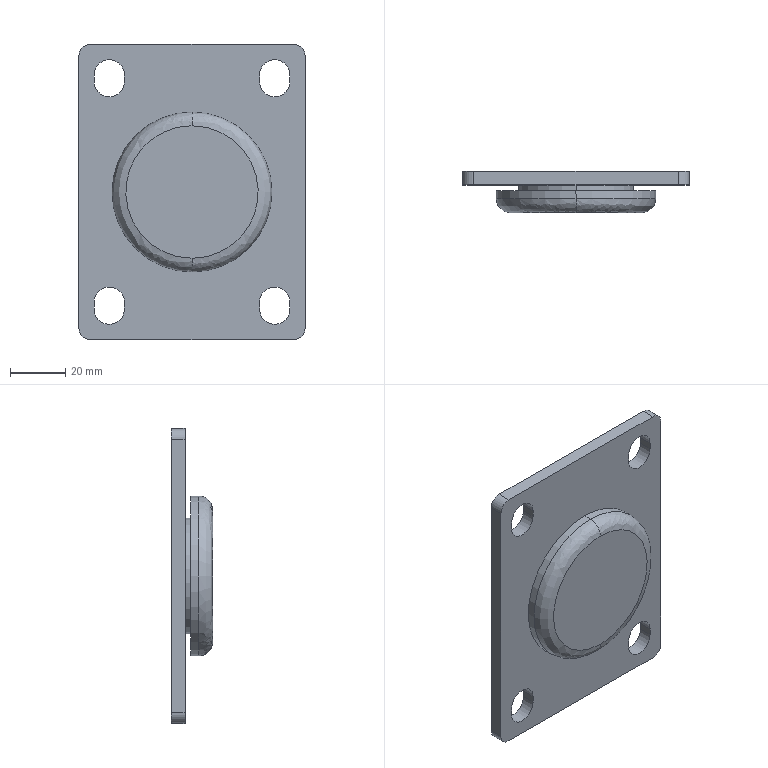Part | SolidWorks | features BaseBody 1 | 1 solid | 47 faces | box 82 x 15 x 107 mm | volume 61600 mm3 | cylinder 26 | plane 19 | spline 2 | commonest cylinder face diameters 11 x12 8 x4 25 x2 40 x2 42 x2 58 x2
STEP:
#1=CARTESIAN_POINT('',(0.,49.,-55.));
#2=VERTEX_POINT('',#1);
#3=CARTESIAN_POINT('',(0.,49.,3.));
#4=VERTEX_POINT('',#3);
#5=CARTESIAN_POINT('',(0.,49.,-26.));
#6=DIRECTION('',(0.,1.,0.));
#7=DIRECTION('',(0.,0.,1.));
#8=AXIS2_PLACEMENT_3D('',#5,#6,#7);
#9=CIRCLE('',#8,29.);
#10=EDGE_CURVE('',#2,#4,#9,.T.);
#11=ORIENTED_EDGE('',*,*,#10,.F.);
#12=CARTESIAN_POINT('',(0.,44.,-50.));
#13=VERTEX_POINT('',#12);
#14=CARTESIAN_POINT('',(0.,49.,-50.));
#15=DIRECTION('',(-1.,0.,0.));
#16=DIRECTION('',(0.,0.,-1.));
#17=AXIS2_PLACEMENT_3D('',#14,#15,#16);
#18=CIRCLE('',#17,5.);
#19=EDGE_CURVE('',#2,#13,#18,.T.);
#20=ORIENTED_EDGE('',*,*,#19,.T.);
#21=CARTESIAN_POINT('',(0.,44.,-2.));
#22=VERTEX_POINT('',#21);
#23=CARTESIAN_POINT('',(0.,44.,-50.));
#24=CARTESIAN_POINT('',(-48.,44.,-50.));
#25=CARTESIAN_POINT('',(-48.,44.,-2.));
#26=CARTESIAN_POINT('',(0.,44.,-2.));
#27=(BOUNDED_CURVE()B_SPLINE_CURVE(3,(#23,#24,#25,#26),.UNSPECIFIED.,.F.,.T.)B_SPLINE_CURVE_WITH_KNOTS((4,4),(0.5,1.),.UNSPECIFIED.)CURVE()GEOMETRIC_REPRESENTATION_ITEM()RATIONAL_B_SPLINE_CURVE((1.,0.3333,0.3333,1.))REPRESENTATION_ITEM(''));
#28=EDGE_CURVE('',#13,#22,#27,.T.);
#29=ORIENTED_EDGE('',*,*,#28,.T.);
#30=CARTESIAN_POINT('',(0.,49.,-2.));
#31=DIRECTION('',(1.,0.,0.));
#32=DIRECTION('',(0.,0.,1.));
#33=AXIS2_PLACEMENT_3D('',#30,#31,#32);
#34=CIRCLE('',#33,5.);
#35=EDGE_CURVE('',#4,#22,#34,.T.);
#36=ORIENTED_EDGE('',*,*,#35,.F.);
#37=EDGE_LOOP('',(#11,#20,#29,#36));
#38=FACE_OUTER_BOUND('',#37,.T.);
#39=CARTESIAN_POINT('',(0.,49.,-55.));
#40=CARTESIAN_POINT('',(-58.,49.,-55.));
#41=CARTESIAN_POINT('',(-58.,49.,3.));
#42=CARTESIAN_POINT('',(0.,49.,3.));
#43=CARTESIAN_POINT('',(0.,46.071,-55.));
#44=CARTESIAN_POINT('',(-58.,46.071,-55.));
#45=CARTESIAN_POINT('',(-58.,46.071,3.));
#46=CARTESIAN_POINT('',(0.,46.071,3.));
#47=CARTESIAN_POINT('',(0.,44.,-52.929));
#48=CARTESIAN_POINT('',(-53.858,44.,-52.929));
#49=CARTESIAN_POINT('',(-53.858,44.,0.9289));
#50=CARTESIAN_POINT('',(0.,44.,0.9289));
#51=CARTESIAN_POINT('',(0.,44.,-50.));
#52=CARTESIAN_POINT('',(-48.,44.,-50.));
#53=CARTESIAN_POINT('',(-48.,44.,-2.));
#54=CARTESIAN_POINT('',(0.,44.,-2.));
#55=(BOUNDED_SURFACE()B_SPLINE_SURFACE(3,3,((#39,#40,#41,#42),(#43,#44,#45,#46),(#47,#48,#49,#50),(#51,#52,#53,#54)),.UNSPECIFIED.,.F.,.F.,.F.)B_SPLINE_SURFACE_WITH_KNOTS((4,4),(4,4),(0.,1.),(0.,1.),.UNSPECIFIED.)GEOMETRIC_REPRESENTATION_ITEM()RATIONAL_B_SPLINE_SURFACE(((1.,0.3333,0.3333,1.),(0.8047,0.2682,0.2682,0.8047),(0.8047,0.2682,0.2682,0.8047),(1.,0.3333,0.3333,1.)))REPRESENTATION_ITEM('')SURFACE());
#56=ADVANCED_FACE('',(#38),#55,.T.);
#57=CARTESIAN_POINT('',(35.5,54.,-66.));
#58=VERTEX_POINT('',#57);
#59=CARTESIAN_POINT('',(30.,54.,-60.5));
#60=VERTEX_POINT('',#59);
#61=CARTESIAN_POINT('',(30.,54.,-66.));
#62=DIRECTION('',(0.,-1.,0.));
#63=DIRECTION('',(0.,0.,1.));
#64=AXIS2_PLACEMENT_3D('',#61,#62,#63);
#65=CIRCLE('',#64,5.5);
#66=EDGE_CURVE('',#58,#60,#65,.T.);
#67=ORIENTED_EDGE('',*,*,#66,.T.);
#68=CARTESIAN_POINT('',(30.,59.,-60.5));
#69=VERTEX_POINT('',#68);
#70=CARTESIAN_POINT('',(30.,54.,-60.5));
#71=DIRECTION('',(0.,1.,0.));
#72=VECTOR('',#71,1000.);
#73=LINE('',#70,#72);
#74=EDGE_CURVE('',#60,#69,#73,.T.);
#75=ORIENTED_EDGE('',*,*,#74,.T.);
#76=CARTESIAN_POINT('',(35.5,59.,-66.));
#77=VERTEX_POINT('',#76);
#78=CARTESIAN_POINT('',(30.,59.,-66.));
#79=DIRECTION('',(0.,-1.,0.));
#80=DIRECTION('',(0.,0.,1.));
#81=AXIS2_PLACEMENT_3D('',#78,#79,#80);
#82=CIRCLE('',#81,5.5);
#83=EDGE_CURVE('',#77,#69,#82,.T.);
#84=ORIENTED_EDGE('',*,*,#83,.F.);
#85=CARTESIAN_POINT('',(35.5,54.,-66.));
#86=DIRECTION('',(0.,1.,0.));
#87=VECTOR('',#86,1000.);
#88=LINE('',#85,#87);
#89=EDGE_CURVE('',#58,#77,#88,.T.);
#90=ORIENTED_EDGE('',*,*,#89,.F.);
#91=EDGE_LOOP('',(#67,#75,#84,#90));
#92=FACE_OUTER_BOUND('',#91,.T.);
#93=CARTESIAN_POINT('',(30.,54.,-66.));
#94=DIRECTION('',(0.,1.,0.));
#95=DIRECTION('',(0.,0.,1.));
#96=AXIS2_PLACEMENT_3D('',#93,#94,#95);
#97=CYLINDRICAL_SURFACE('',#96,5.5);
#98=ADVANCED_FACE('',(#92),#97,.F.);
#99=CARTESIAN_POINT('',(35.5,54.,16.5));
#100=VERTEX_POINT('',#99);
#101=CARTESIAN_POINT('',(30.,54.,22.));
#102=VERTEX_POINT('',#101);
#103=CARTESIAN_POINT('',(30.,54.,16.5));
#104=DIRECTION('',(0.,-1.,0.));
#105=DIRECTION('',(0.,0.,1.));
#106=AXIS2_PLACEMENT_3D('',#103,#104,#105);
#107=CIRCLE('',#106,5.5);
#108=EDGE_CURVE('',#100,#102,#107,.T.);
#109=ORIENTED_EDGE('',*,*,#108,.T.);
#110=CARTESIAN_POINT('',(30.,59.,22.));
#111=VERTEX_POINT('',#110);
#112=CARTESIAN_POINT('',(30.,54.,22.));
#113=DIRECTION('',(0.,1.,0.));
#114=VECTOR('',#113,1000.);
#115=LINE('',#112,#114);
#116=EDGE_CURVE('',#102,#111,#115,.T.);
#117=ORIENTED_EDGE('',*,*,#116,.T.);
#118=CARTESIAN_POINT('',(35.5,59.,16.5));
#119=VERTEX_POINT('',#118);
#120=CARTESIAN_POINT('',(30.,59.,16.5));
#121=DIRECTION('',(0.,-1.,0.));
#122=DIRECTION('',(0.,0.,1.));
#123=AXIS2_PLACEMENT_3D('',#120,#121,#122);
#124=CIRCLE('',#123,5.5);
#125=EDGE_CURVE('',#119,#111,#124,.T.);
#126=ORIENTED_EDGE('',*,*,#125,.F.);
#127=CARTESIAN_POINT('',(35.5,54.,16.5));
#128=DIRECTION('',(0.,1.,0.));
#129=VECTOR('',#128,1000.);
#130=LINE('',#127,#129);
#131=EDGE_CURVE('',#100,#119,#130,.T.);
#132=ORIENTED_EDGE('',*,*,#131,.F.);
#133=EDGE_LOOP('',(#109,#117,#126,#132));
#134=FACE_OUTER_BOUND('',#133,.T.);
#135=CARTESIAN_POINT('',(30.,54.,16.5));
#136=DIRECTION('',(0.,1.,0.));
#137=DIRECTION('',(0.,0.,1.));
#138=AXIS2_PLACEMENT_3D('',#135,#136,#137);
#139=CYLINDRICAL_SURFACE('',#138,5.5);
#140=ADVANCED_FACE('',(#134),#139,.F.);
#141=CARTESIAN_POINT('',(-24.5,54.,-66.));
#142=VERTEX_POINT('',#141);
#143=CARTESIAN_POINT('',(-30.,54.,-60.5));
#144=VERTEX_POINT('',#143);
#145=CARTESIAN_POINT('',(-30.,54.,-66.));
#146=DIRECTION('',(0.,-1.,0.));
#147=DIRECTION('',(0.,0.,1.));
#148=AXIS2_PLACEMENT_3D('',#145,#146,#147);
#149=CIRCLE('',#148,5.5);
#150=EDGE_CURVE('',#142,#144,#149,.T.);
#151=ORIENTED_EDGE('',*,*,#150,.T.);
#152=CARTESIAN_POINT('',(-30.,59.,-60.5));
#153=VERTEX_POINT('',#152);
#154=CARTESIAN_POINT('',(-30.,54.,-60.5));
#155=DIRECTION('',(0.,1.,0.));
#156=VECTOR('',#155,1000.);
#157=LINE('',#154,#156);
#158=EDGE_CURVE('',#144,#153,#157,.T.);
#159=ORIENTED_EDGE('',*,*,#158,.T.);
#160=CARTESIAN_POINT('',(-24.5,59.,-66.));
#161=VERTEX_POINT('',#160);
#162=CARTESIAN_POINT('',(-30.,59.,-66.));
#163=DIRECTION('',(0.,-1.,0.));
#164=DIRECTION('',(0.,0.,1.));
#165=AXIS2_PLACEMENT_3D('',#162,#163,#164);
#166=CIRCLE('',#165,5.5);
#167=EDGE_CURVE('',#161,#153,#166,.T.);
#168=ORIENTED_EDGE('',*,*,#167,.F.);
#169=CARTESIAN_POINT('',(-24.5,54.,-66.));
#170=DIRECTION('',(0.,1.,0.));
#171=VECTOR('',#170,1000.);
#172=LINE('',#169,#171);
#173=EDGE_CURVE('',#142,#161,#172,.T.);
#174=ORIENTED_EDGE('',*,*,#173,.F.);
#175=EDGE_LOOP('',(#151,#159,#168,#174));
#176=FACE_OUTER_BOUND('',#175,.T.);
#177=CARTESIAN_POINT('',(-30.,54.,-66.));
#178=DIRECTION('',(0.,1.,0.));
#179=DIRECTION('',(0.,0.,1.));
#180=AXIS2_PLACEMENT_3D('',#177,#178,#179);
#181=CYLINDRICAL_SURFACE('',#180,5.5);
#182=ADVANCED_FACE('',(#176),#181,.F.);
#183=CARTESIAN_POINT('',(-24.5,54.,16.5));
#184=VERTEX_POINT('',#183);
#185=CARTESIAN_POINT('',(-30.,54.,22.));
#186=VERTEX_POINT('',#185);
#187=CARTESIAN_POINT('',(-30.,54.,16.5));
#188=DIRECTION('',(0.,-1.,0.));
#189=DIRECTION('',(0.,0.,1.));
#190=AXIS2_PLACEMENT_3D('',#187,#188,#189);
#191=CIRCLE('',#190,5.5);
#192=EDGE_CURVE('',#184,#186,#191,.T.);
#193=ORIENTED_EDGE('',*,*,#192,.T.);
#194=CARTESIAN_POINT('',(-30.,59.,22.));
#195=VERTEX_POINT('',#194);
#196=CARTESIAN_POINT('',(-30.,54.,22.));
#197=DIRECTION('',(0.,1.,0.));
#198=VECTOR('',#197,1000.);
#199=LINE('',#196,#198);
#200=EDGE_CURVE('',#186,#195,#199,.T.);
#201=ORIENTED_EDGE('',*,*,#200,.T.);
#202=CARTESIAN_POINT('',(-24.5,59.,16.5));
#203=VERTEX_POINT('',#202);
#204=CARTESIAN_POINT('',(-30.,59.,16.5));
#205=DIRECTION('',(0.,-1.,0.));
#206=DIRECTION('',(0.,0.,1.));
#207=AXIS2_PLACEMENT_3D('',#204,#205,#206);
#208=CIRCLE('',#207,5.5);
#209=EDGE_CURVE('',#203,#195,#208,.T.);
#210=ORIENTED_EDGE('',*,*,#209,.F.);
#211=CARTESIAN_POINT('',(-24.5,54.,16.5));
#212=DIRECTION('',(0.,1.,0.));
#213=VECTOR('',#212,1000.);
#214=LINE('',#211,#213);
#215=EDGE_CURVE('',#184,#203,#214,.T.);
#216=ORIENTED_EDGE('',*,*,#215,.F.);
#217=EDGE_LOOP('',(#193,#201,#210,#216));
#218=FACE_OUTER_BOUND('',#217,.T.);
#219=CARTESIAN_POINT('',(-30.,54.,16.5));
#220=DIRECTION('',(0.,1.,0.));
#221=DIRECTION('',(0.,0.,1.));
#222=AXIS2_PLACEMENT_3D('',#219,#220,#221);
#223=CYLINDRICAL_SURFACE('',#222,5.5);
#224=ADVANCED_FACE('',(#218),#223,.F.);
#225=CARTESIAN_POINT('',(0.,52.,-5.));
#226=VERTEX_POINT('',#225);
#227=CARTESIAN_POINT('',(0.,52.,-47.));
#228=VERTEX_POINT('',#227);
#229=CARTESIAN_POINT('',(0.,52.,-26.));
#230=DIRECTION('',(0.,1.,0.));
#231=DIRECTION('',(0.,0.,1.));
#232=AXIS2_PLACEMENT_3D('',#229,#230,#231);
#233=CIRCLE('',#232,21.);
#234=EDGE_CURVE('',#226,#228,#233,.T.);
#235=ORIENTED_EDGE('',*,*,#234,.T.);
#236=CARTESIAN_POINT('',(0.,54.,-47.));
#237=VERTEX_POINT('',#236);
#238=CARTESIAN_POINT('',(0.,52.,-47.));
#239=DIRECTION('',(0.,1.,0.));
#240=VECTOR('',#239,1000.);
#241=LINE('',#238,#240);
#242=EDGE_CURVE('',#228,#237,#241,.T.);
#243=ORIENTED_EDGE('',*,*,#242,.T.);
#244=CARTESIAN_POINT('',(0.,54.,-5.));
#245=VERTEX_POINT('',#244);
#246=CARTESIAN_POINT('',(0.,54.,-26.));
#247=DIRECTION('',(0.,-1.,0.));
#248=DIRECTION('',(0.,0.,1.));
#249=AXIS2_PLACEMENT_3D('',#246,#247,#248);
#250=CIRCLE('',#249,21.);
#251=EDGE_CURVE('',#237,#245,#250,.T.);
#252=ORIENTED_EDGE('',*,*,#251,.T.);
#253=CARTESIAN_POINT('',(0.,52.,-5.));
#254=DIRECTION('',(0.,1.,0.));
#255=VECTOR('',#254,1000.);
#256=LINE('',#253,#255);
#257=EDGE_CURVE('',#226,#245,#256,.T.);
#258=ORIENTED_EDGE('',*,*,#257,.F.);
#259=EDGE_LOOP('',(#235,#243,#252,#258));
#260=FACE_OUTER_BOUND('',#259,.T.);
#261=CARTESIAN_POINT('',(0.,52.,-26.));
#262=DIRECTION('',(0.,1.,0.));
#263=DIRECTION('',(0.,0.,1.));
#264=AXIS2_PLACEMENT_3D('',#261,#262,#263);
#265=CYLINDRICAL_SURFACE('',#264,21.);
#266=ADVANCED_FACE('',(#260),#265,.T.);
#267=CARTESIAN_POINT('',(0.,58.,-56.));
#268=VERTEX_POINT('',#267);
#269=CARTESIAN_POINT('',(0.,58.,4.));
#270=VERTEX_POINT('',#269);
#271=CARTESIAN_POINT('',(0.,58.,-26.));
#272=DIRECTION('',(0.,1.,0.));
#273=DIRECTION('',(0.,0.,1.));
#274=AXIS2_PLACEMENT_3D('',#271,#272,#273);
#275=CIRCLE('',#274,30.);
#276=EDGE_CURVE('',#268,#270,#275,.T.);
#277=ORIENTED_EDGE('',*,*,#276,.F.);
#278=CARTESIAN_POINT('',(0.,59.,-56.));
#279=VERTEX_POINT('',#278);
#280=CARTESIAN_POINT('',(0.,58.,-56.));
#281=DIRECTION('',(0.,1.,0.));
#282=VECTOR('',#281,1000.);
#283=LINE('',#280,#282);
#284=EDGE_CURVE('',#268,#279,#283,.T.);
#285=ORIENTED_EDGE('',*,*,#284,.T.);
#286=CARTESIAN_POINT('',(0.,59.,4.));
#287=VERTEX_POINT('',#286);
#288=CARTESIAN_POINT('',(0.,59.,-26.));
#289=DIRECTION('',(0.,-1.,0.));
#290=DIRECTION('',(0.,0.,1.));
#291=AXIS2_PLACEMENT_3D('',#288,#289,#290);
#292=CIRCLE('',#291,30.);
#293=EDGE_CURVE('',#287,#279,#292,.T.);
#294=ORIENTED_EDGE('',*,*,#293,.F.);
#295=CARTESIAN_POINT('',(0.,58.,4.));
#296=DIRECTION('',(0.,1.,0.));
#297=VECTOR('',#296,1000.);
#298=LINE('',#295,#297);
#299=EDGE_CURVE('',#270,#287,#298,.T.);
#300=ORIENTED_EDGE('',*,*,#299,.F.);
#301=EDGE_LOOP('',(#277,#285,#294,#300));
#302=FACE_OUTER_BOUND('',#301,.T.);
#303=CARTESIAN_POINT('',(0.,58.,-26.));
#304=DIRECTION('',(0.,1.,0.));
#305=DIRECTION('',(0.,0.,1.));
#306=AXIS2_PLACEMENT_3D('',#303,#304,#305);
#307=CYLINDRICAL_SURFACE('',#306,30.);
#308=ADVANCED_FACE('',(#302),#307,.F.);
#309=CARTESIAN_POINT('',(0.,49.,-26.));
#310=DIRECTION('',(0.,1.,0.));
#311=DIRECTION('',(0.,0.,1.));
#312=AXIS2_PLACEMENT_3D('',#309,#310,#311);
#313=CIRCLE('',#312,29.);
#314=EDGE_CURVE('',#4,#2,#313,.T.);
#315=ORIENTED_EDGE('',*,*,#314,.T.);
#316=CARTESIAN_POINT('',(0.,52.,-55.));
#317=VERTEX_POINT('',#316);
#318=CARTESIAN_POINT('',(0.,52.,-55.));
#319=DIRECTION('',(0.,1.,0.));
#320=VECTOR('',#319,1000.);
#321=LINE('',#318,#320);
#322=EDGE_CURVE('',#2,#317,#321,.T.);
#323=ORIENTED_EDGE('',*,*,#322,.T.);
#324=CARTESIAN_POINT('',(0.,52.,3.));
#325=VERTEX_POINT('',#324);
#326=CARTESIAN_POINT('',(0.,52.,-26.));
#327=DIRECTION('',(0.,-1.,0.));
#328=DIRECTION('',(0.,0.,1.));
#329=AXIS2_PLACEMENT_3D('',#326,#327,#328);
#330=CIRCLE('',#329,29.);
#331=EDGE_CURVE('',#317,#325,#330,.T.);
#332=ORIENTED_EDGE('',*,*,#331,.T.);
#333=CARTESIAN_POINT('',(0.,52.,3.));
#334=DIRECTION('',(0.,1.,0.));
#335=VECTOR('',#334,1000.);
#336=LINE('',#333,#335);
#337=EDGE_CURVE('',#4,#325,#336,.T.);
#338=ORIENTED_EDGE('',*,*,#337,.F.);
#339=EDGE_LOOP('',(#315,#323,#332,#338));
#340=FACE_OUTER_BOUND('',#339,.T.);
#341=CARTESIAN_POINT('',(0.,52.,-26.));
#342=DIRECTION('',(0.,1.,0.));
#343=DIRECTION('',(0.,0.,1.));
#344=AXIS2_PLACEMENT_3D('',#341,#342,#343);
#345=CYLINDRICAL_SURFACE('',#344,29.);
#346=ADVANCED_FACE('',(#340),#345,.T.);
#347=CARTESIAN_POINT('',(0.,57.5,-46.));
#348=VERTEX_POINT('',#347);
#349=CARTESIAN_POINT('',(0.,57.5,-6.));
#350=VERTEX_POINT('',#349);
#351=CARTESIAN_POINT('',(0.,57.5,-26.));
#352=DIRECTION('',(0.,1.,0.));
#353=DIRECTION('',(0.,0.,1.));
#354=AXIS2_PLACEMENT_3D('',#351,#352,#353);
#355=CIRCLE('',#354,20.);
#356=EDGE_CURVE('',#348,#350,#355,.T.);
#357=ORIENTED_EDGE('',*,*,#356,.F.);
#358=CARTESIAN_POINT('',(0.,58.,-46.));
#359=VERTEX_POINT('',#358);
#360=CARTESIAN_POINT('',(0.,57.5,-46.));
#361=DIRECTION('',(0.,1.,0.));
#362=VECTOR('',#361,1000.);
#363=LINE('',#360,#362);
#364=EDGE_CURVE('',#348,#359,#363,.T.);
#365=ORIENTED_EDGE('',*,*,#364,.T.);
#366=CARTESIAN_POINT('',(0.,58.,-6.));
#367=VERTEX_POINT('',#366);
#368=CARTESIAN_POINT('',(0.,58.,-26.));
#369=DIRECTION('',(0.,-1.,0.));
#370=DIRECTION('',(0.,0.,1.));
#371=AXIS2_PLACEMENT_3D('',#368,#369,#370);
#372=CIRCLE('',#371,20.);
#373=EDGE_CURVE('',#367,#359,#372,.T.);
#374=ORIENTED_EDGE('',*,*,#373,.F.);
#375=CARTESIAN_POINT('',(0.,57.5,-6.));
#376=DIRECTION('',(0.,1.,0.));
#377=VECTOR('',#376,1000.);
#378=LINE('',#375,#377);
#379=EDGE_CURVE('',#350,#367,#378,.T.);
#380=ORIENTED_EDGE('',*,*,#379,.F.);
#381=EDGE_LOOP('',(#357,#365,#374,#380));
#382=FACE_OUTER_BOUND('',#381,.T.);
#383=CARTESIAN_POINT('',(0.,57.5,-26.));
#384=DIRECTION('',(0.,1.,0.));
#385=DIRECTION('',(0.,0.,1.));
#386=AXIS2_PLACEMENT_3D('',#383,#384,#385);
#387=CYLINDRICAL_SURFACE('',#386,20.);
#388=ADVANCED_FACE('',(#382),#387,.F.);
#389=CARTESIAN_POINT('',(0.,57.5,-38.5));
#390=VERTEX_POINT('',#389);
#391=CARTESIAN_POINT('',(0.,57.5,-13.5));
#392=VERTEX_POINT('',#391);
#393=CARTESIAN_POINT('',(0.,57.5,-26.));
#394=DIRECTION('',(0.,-1.,0.));
#395=DIRECTION('',(0.,0.,1.));
#396=AXIS2_PLACEMENT_3D('',#393,#394,#395);
#397=CIRCLE('',#396,12.5);
#398=EDGE_CURVE('',#390,#392,#397,.T.);
#399=ORIENTED_EDGE('',*,*,#398,.F.);
#400=CARTESIAN_POINT('',(0.,59.,-38.5));
#401=VERTEX_POINT('',#400);
#402=CARTESIAN_POINT('',(0.,56.5,-38.5));
#403=DIRECTION('',(0.,1.,0.));
#404=VECTOR('',#403,1000.);
#405=LINE('',#402,#404);
#406=EDGE_CURVE('',#390,#401,#405,.T.);
#407=ORIENTED_EDGE('',*,*,#406,.T.);
#408=CARTESIAN_POINT('',(0.,59.,-13.5));
#409=VERTEX_POINT('',#408);
#410=CARTESIAN_POINT('',(0.,59.,-26.));
#411=DIRECTION('',(0.,-1.,0.));
#412=DIRECTION('',(0.,0.,1.));
#413=AXIS2_PLACEMENT_3D('',#410,#411,#412);
#414=CIRCLE('',#413,12.5);
#415=EDGE_CURVE('',#401,#409,#414,.T.);
#416=ORIENTED_EDGE('',*,*,#415,.T.);
#417=CARTESIAN_POINT('',(0.,56.5,-13.5));
#418=DIRECTION('',(0.,1.,0.));
#419=VECTOR('',#418,1000.);
#420=LINE('',#417,#419);
#421=EDGE_CURVE('',#392,#409,#420,.T.);
#422=ORIENTED_EDGE('',*,*,#421,.F.);
#423=EDGE_LOOP('',(#399,#407,#416,#422));
#424=FACE_OUTER_BOUND('',#423,.T.);
#425=CARTESIAN_POINT('',(0.,56.5,-26.));
#426=DIRECTION('',(0.,1.,0.));
#427=DIRECTION('',(0.,0.,1.));
#428=AXIS2_PLACEMENT_3D('',#425,#426,#427);
#429=CYLINDRICAL_SURFACE('',#428,12.5);
#430=ADVANCED_FACE('',(#424),#429,.T.);
#431=CARTESIAN_POINT('',(-37.,54.,-79.5));
#432=VERTEX_POINT('',#431);
#433=CARTESIAN_POINT('',(-41.,54.,-75.5));
#434=VERTEX_POINT('',#433);
#435=CARTESIAN_POINT('',(-37.,54.,-75.5));
#436=DIRECTION('',(0.,1.,0.));
#437=DIRECTION('',(0.,0.,1.));
#438=AXIS2_PLACEMENT_3D('',#435,#436,#437);
#439=CIRCLE('',#438,4.);
#440=EDGE_CURVE('',#432,#434,#439,.T.);
#441=ORIENTED_EDGE('',*,*,#440,.F.);
#442=CARTESIAN_POINT('',(37.,54.,-79.5));
#443=VERTEX_POINT('',#442);
#444=CARTESIAN_POINT('',(-37.,54.,-79.5));
#445=DIRECTION('',(-1.,0.,0.));
#446=VECTOR('',#445,1000.);
#447=LINE('',#444,#446);
#448=EDGE_CURVE('',#443,#432,#447,.T.);
#449=ORIENTED_EDGE('',*,*,#448,.F.);
#450=CARTESIAN_POINT('',(41.,54.,-75.5));
#451=VERTEX_POINT('',#450);
#452=CARTESIAN_POINT('',(37.,54.,-75.5));
#453=DIRECTION('',(0.,1.,0.));
#454=DIRECTION('',(0.,0.,1.));
#455=AXIS2_PLACEMENT_3D('',#452,#453,#454);
#456=CIRCLE('',#455,4.);
#457=EDGE_CURVE('',#451,#443,#456,.T.);
#458=ORIENTED_EDGE('',*,*,#457,.F.);
#459=CARTESIAN_POINT('',(41.,54.,23.5));
#460=VERTEX_POINT('',#459);
#461=CARTESIAN_POINT('',(41.,54.,23.5));
#462=DIRECTION('',(0.,0.,-1.));
#463=VECTOR('',#462,1000.);
#464=LINE('',#461,#463);
#465=EDGE_CURVE('',#460,#451,#464,.T.);
#466=ORIENTED_EDGE('',*,*,#465,.F.);
#467=CARTESIAN_POINT('',(37.,54.,27.5));
#468=VERTEX_POINT('',#467);
#469=CARTESIAN_POINT('',(37.,54.,23.5));
#470=DIRECTION('',(0.,1.,0.));
#471=DIRECTION('',(0.,0.,1.));
#472=AXIS2_PLACEMENT_3D('',#469,#470,#471);
#473=CIRCLE('',#472,4.);
#474=EDGE_CURVE('',#468,#460,#473,.T.);
#475=ORIENTED_EDGE('',*,*,#474,.F.);
#476=CARTESIAN_POINT('',(-37.,54.,27.5));
#477=VERTEX_POINT('',#476);
#478=CARTESIAN_POINT('',(-37.,54.,27.5));
#479=DIRECTION('',(1.,0.,0.));
#480=VECTOR('',#479,1000.);
#481=LINE('',#478,#480);
#482=EDGE_CURVE('',#477,#468,#481,.T.);
#483=ORIENTED_EDGE('',*,*,#482,.F.);
#484=CARTESIAN_POINT('',(-41.,54.,23.5));
#485=VERTEX_POINT('',#484);
#486=CARTESIAN_POINT('',(-37.,54.,23.5));
#487=DIRECTION('',(0.,1.,0.));
#488=DIRECTION('',(0.,0.,1.));
#489=AXIS2_PLACEMENT_3D('',#486,#487,#488);
#490=CIRCLE('',#489,4.);
#491=EDGE_CURVE('',#485,#477,#490,.T.);
#492=ORIENTED_EDGE('',*,*,#491,.F.);
#493=CARTESIAN_POINT('',(-41.,54.,23.5));
#494=DIRECTION('',(0.,0.,1.));
#495=VECTOR('',#494,1000.);
#496=LINE('',#493,#495);
#497=EDGE_CURVE('',#434,#485,#496,.T.);
#498=ORIENTED_EDGE('',*,*,#497,.F.);
#499=EDGE_LOOP('',(#441,#449,#458,#466,#475,#483,#492,#498));
#500=FACE_OUTER_BOUND('',#499,.T.);
#501=CARTESIAN_POINT('',(24.5,54.,-66.));
#502=VERTEX_POINT('',#501);
#503=CARTESIAN_POINT('',(24.5,54.,-68.5));
#504=VERTEX_POINT('',#503);
#505=CARTESIAN_POINT('',(24.5,54.,23.5));
#506=DIRECTION('',(0.,0.,-1.));
#507=VECTOR('',#506,1000.);
#508=LINE('',#505,#507);
#509=EDGE_CURVE('',#502,#504,#508,.T.);
#510=ORIENTED_EDGE('',*,*,#509,.F.);
#511=CARTESIAN_POINT('',(30.,54.,-66.));
#512=DIRECTION('',(0.,-1.,0.));
#513=DIRECTION('',(0.,0.,1.));
#514=AXIS2_PLACEMENT_3D('',#511,#512,#513);
#515=CIRCLE('',#514,5.5);
#516=EDGE_CURVE('',#60,#502,#515,.T.);
#517=ORIENTED_EDGE('',*,*,#516,.F.);
#518=ORIENTED_EDGE('',*,*,#66,.F.);
#519=CARTESIAN_POINT('',(35.5,54.,-68.5));
#520=VERTEX_POINT('',#519);
#521=CARTESIAN_POINT('',(35.5,54.,23.5));
#522=DIRECTION('',(0.,0.,1.));
#523=VECTOR('',#522,1000.);
#524=LINE('',#521,#523);
#525=EDGE_CURVE('',#520,#58,#524,.T.);
#526=ORIENTED_EDGE('',*,*,#525,.F.);
#527=CARTESIAN_POINT('',(30.,54.,-68.5));
#528=DIRECTION('',(0.,-1.,0.));
#529=DIRECTION('',(0.,0.,1.));
#530=AXIS2_PLACEMENT_3D('',#527,#528,#529);
#531=CIRCLE('',#530,5.5);
#532=EDGE_CURVE('',#504,#520,#531,.T.);
#533=ORIENTED_EDGE('',*,*,#532,.F.);
#534=EDGE_LOOP('',(#510,#517,#518,#526,#533));
#535=FACE_BOUND('',#534,.T.);
#536=ORIENTED_EDGE('',*,*,#108,.F.);
#537=CARTESIAN_POINT('',(35.5,54.,14.));
#538=VERTEX_POINT('',#537);
#539=CARTESIAN_POINT('',(35.5,54.,23.5));
#540=DIRECTION('',(0.,0.,1.));
#541=VECTOR('',#540,1000.);
#542=LINE('',#539,#541);
#543=EDGE_CURVE('',#538,#100,#542,.T.);
#544=ORIENTED_EDGE('',*,*,#543,.F.);
#545=CARTESIAN_POINT('',(24.5,54.,14.));
#546=VERTEX_POINT('',#545);
#547=CARTESIAN_POINT('',(30.,54.,14.));
#548=DIRECTION('',(0.,-1.,0.));
#549=DIRECTION('',(0.,0.,1.));
#550=AXIS2_PLACEMENT_3D('',#547,#548,#549);
#551=CIRCLE('',#550,5.5);
#552=EDGE_CURVE('',#546,#538,#551,.T.);
#553=ORIENTED_EDGE('',*,*,#552,.F.);
#554=CARTESIAN_POINT('',(24.5,54.,16.5));
#555=VERTEX_POINT('',#554);
#556=CARTESIAN_POINT('',(24.5,54.,23.5));
#557=DIRECTION('',(0.,0.,-1.));
#558=VECTOR('',#557,1000.);
#559=LINE('',#556,#558);
#560=EDGE_CURVE('',#555,#546,#559,.T.);
#561=ORIENTED_EDGE('',*,*,#560,.F.);
#562=CARTESIAN_POINT('',(30.,54.,16.5));
#563=DIRECTION('',(0.,-1.,0.));
#564=DIRECTION('',(0.,0.,1.));
#565=AXIS2_PLACEMENT_3D('',#562,#563,#564);
#566=CIRCLE('',#565,5.5);
#567=EDGE_CURVE('',#102,#555,#566,.T.);
#568=ORIENTED_EDGE('',*,*,#567,.F.);
#569=EDGE_LOOP('',(#536,#544,#553,#561,#568));
#570=FACE_BOUND('',#569,.T.);
#571=CARTESIAN_POINT('',(-35.5,54.,-66.));
#572=VERTEX_POINT('',#571);
#573=CARTESIAN_POINT('',(-35.5,54.,-68.5));
#574=VERTEX_POINT('',#573);
#575=CARTESIAN_POINT('',(-35.5,54.,23.5));
#576=DIRECTION('',(0.,0.,-1.));
#577=VECTOR('',#576,1000.);
#578=LINE('',#575,#577);
#579=EDGE_CURVE('',#572,#574,#578,.T.);
#580=ORIENTED_EDGE('',*,*,#579,.F.);
#581=CARTESIAN_POINT('',(-30.,54.,-66.));
#582=DIRECTION('',(0.,-1.,0.));
#583=DIRECTION('',(0.,0.,1.));
#584=AXIS2_PLACEMENT_3D('',#581,#582,#583);
#585=CIRCLE('',#584,5.5);
#586=EDGE_CURVE('',#144,#572,#585,.T.);
#587=ORIENTED_EDGE('',*,*,#586,.F.);
#588=ORIENTED_EDGE('',*,*,#150,.F.);
#589=CARTESIAN_POINT('',(-24.5,54.,-68.5));
#590=VERTEX_POINT('',#589);
#591=CARTESIAN_POINT('',(-24.5,54.,23.5));
#592=DIRECTION('',(0.,0.,1.));
#593=VECTOR('',#592,1000.);
#594=LINE('',#591,#593);
#595=EDGE_CURVE('',#590,#142,#594,.T.);
#596=ORIENTED_EDGE('',*,*,#595,.F.);
#597=CARTESIAN_POINT('',(-30.,54.,-68.5));
#598=DIRECTION('',(0.,-1.,0.));
#599=DIRECTION('',(0.,0.,1.));
#600=AXIS2_PLACEMENT_3D('',#597,#598,#599);
#601=CIRCLE('',#600,5.5);
#602=EDGE_CURVE('',#574,#590,#601,.T.);
#603=ORIENTED_EDGE('',*,*,#602,.F.);
#604=EDGE_LOOP('',(#580,#587,#588,#596,#603));
#605=FACE_BOUND('',#604,.T.);
#606=ORIENTED_EDGE('',*,*,#192,.F.);
#607=CARTESIAN_POINT('',(-24.5,54.,14.));
#608=VERTEX_POINT('',#607);
#609=CARTESIAN_POINT('',(-24.5,54.,23.5));
#610=DIRECTION('',(0.,0.,1.));
#611=VECTOR('',#610,1000.);
#612=LINE('',#609,#611);
#613=EDGE_CURVE('',#608,#184,#612,.T.);
#614=ORIENTED_EDGE('',*,*,#613,.F.);
#615=CARTESIAN_POINT('',(-35.5,54.,14.));
#616=VERTEX_POINT('',#615);
#617=CARTESIAN_POINT('',(-30.,54.,14.));
#618=DIRECTION('',(0.,-1.,0.));
#619=DIRECTION('',(0.,0.,1.));
#620=AXIS2_PLACEMENT_3D('',#617,#618,#619);
#621=CIRCLE('',#620,5.5);
#622=EDGE_CURVE('',#616,#608,#621,.T.);
#623=ORIENTED_EDGE('',*,*,#622,.F.);
#624=CARTESIAN_POINT('',(-35.5,54.,16.5));
#625=VERTEX_POINT('',#624);
#626=CARTESIAN_POINT('',(-35.5,54.,23.5));
#627=DIRECTION('',(0.,0.,-1.));
#628=VECTOR('',#627,1000.);
#629=LINE('',#626,#628);
#630=EDGE_CURVE('',#625,#616,#629,.T.);
#631=ORIENTED_EDGE('',*,*,#630,.F.);
#632=CARTESIAN_POINT('',(-30.,54.,16.5));
#633=DIRECTION('',(0.,-1.,0.));
#634=DIRECTION('',(0.,0.,1.));
#635=AXIS2_PLACEMENT_3D('',#632,#633,#634);
#636=CIRCLE('',#635,5.5);
#637=EDGE_CURVE('',#186,#625,#636,.T.);
#638=ORIENTED_EDGE('',*,*,#637,.F.);
#639=EDGE_LOOP('',(#606,#614,#623,#631,#638));
#640=FACE_BOUND('',#639,.T.);
#641=CARTESIAN_POINT('',(0.,54.,-26.));
#642=DIRECTION('',(0.,-1.,0.));
#643=DIRECTION('',(0.,0.,1.));
#644=AXIS2_PLACEMENT_3D('',#641,#642,#643);
#645=CIRCLE('',#644,21.);
#646=EDGE_CURVE('',#245,#237,#645,.T.);
#647=ORIENTED_EDGE('',*,*,#646,.F.);
#648=ORIENTED_EDGE('',*,*,#251,.F.);
#649=EDGE_LOOP('',(#647,#648));
#650=FACE_BOUND('',#649,.T.);
#651=CARTESIAN_POINT('',(-37.,54.,23.5));
#652=DIRECTION('',(0.,1.,0.));
#653=DIRECTION('',(0.,0.,1.));
#654=AXIS2_PLACEMENT_3D('',#651,#652,#653);
#655=PLANE('',#654);
#656=ADVANCED_FACE('',(#500,#535,#570,#605,#640,#650),#655,.F.);
#657=ORIENTED_EDGE('',*,*,#497,.T.);
#658=CARTESIAN_POINT('',(-41.,59.,23.5));
#659=VERTEX_POINT('',#658);
#660=CARTESIAN_POINT('',(-41.,54.,23.5));
#661=DIRECTION('',(0.,1.,0.));
#662=VECTOR('',#661,1000.);
#663=LINE('',#660,#662);
#664=EDGE_CURVE('',#485,#659,#663,.T.);
#665=ORIENTED_EDGE('',*,*,#664,.T.);
#666=CARTESIAN_POINT('',(-41.,59.,-75.5));
#667=VERTEX_POINT('',#666);
#668=CARTESIAN_POINT('',(-41.,59.,-75.5));
#669=DIRECTION('',(0.,0.,-1.));
#670=VECTOR('',#669,1000.);
#671=LINE('',#668,#670);
#672=EDGE_CURVE('',#659,#667,#671,.T.);
#673=ORIENTED_EDGE('',*,*,#672,.T.);
#674=CARTESIAN_POINT('',(-41.,54.,-75.5));
#675=DIRECTION('',(0.,-1.,0.));
#676=VECTOR('',#675,1000.);
#677=LINE('',#674,#676);
#678=EDGE_CURVE('',#667,#434,#677,.T.);
#679=ORIENTED_EDGE('',*,*,#678,.T.);
#680=EDGE_LOOP('',(#657,#665,#673,#679));
#681=FACE_OUTER_BOUND('',#680,.T.);
#682=CARTESIAN_POINT('',(-41.,54.,-75.5));
#683=DIRECTION('',(-1.,0.,0.));
#684=DIRECTION('',(0.,0.,1.));
#685=AXIS2_PLACEMENT_3D('',#682,#683,#684);
#686=PLANE('',#685);
#687=ADVANCED_FACE('',(#681),#686,.T.);
#688=ORIENTED_EDGE('',*,*,#440,.T.);
#689=ORIENTED_EDGE('',*,*,#678,.F.);
#690=CARTESIAN_POINT('',(-37.,59.,-79.5));
#691=VERTEX_POINT('',#690);
#692=CARTESIAN_POINT('',(-37.,59.,-75.5));
#693=DIRECTION('',(0.,-1.,0.));
#694=DIRECTION('',(0.,0.,1.));
#695=AXIS2_PLACEMENT_3D('',#692,#693,#694);
#696=CIRCLE('',#695,4.);
#697=EDGE_CURVE('',#667,#691,#696,.T.);
#698=ORIENTED_EDGE('',*,*,#697,.T.);
#699=CARTESIAN_POINT('',(-37.,54.,-79.5));
#700=DIRECTION('',(0.,-1.,0.));
#701=VECTOR('',#700,1000.);
#702=LINE('',#699,#701);
#703=EDGE_CURVE('',#691,#432,#702,.T.);
#704=ORIENTED_EDGE('',*,*,#703,.T.);
#705=EDGE_LOOP('',(#688,#689,#698,#704));
#706=FACE_OUTER_BOUND('',#705,.T.);
#707=CARTESIAN_POINT('',(-37.,54.,-75.5));
#708=DIRECTION('',(0.,1.,0.));
#709=DIRECTION('',(0.,0.,1.));
#710=AXIS2_PLACEMENT_3D('',#707,#708,#709);
#711=CYLINDRICAL_SURFACE('',#710,4.);
#712=ADVANCED_FACE('',(#706),#711,.T.);
#713=ORIENTED_EDGE('',*,*,#448,.T.);
#714=ORIENTED_EDGE('',*,*,#703,.F.);
#715=CARTESIAN_POINT('',(37.,59.,-79.5));
#716=VERTEX_POINT('',#715);
#717=CARTESIAN_POINT('',(37.,59.,-79.5));
#718=DIRECTION('',(1.,0.,0.));
#719=VECTOR('',#718,1000.);
#720=LINE('',#717,#719);
#721=EDGE_CURVE('',#691,#716,#720,.T.);
#722=ORIENTED_EDGE('',*,*,#721,.T.);
#723=CARTESIAN_POINT('',(37.,54.,-79.5));
#724=DIRECTION('',(0.,-1.,0.));
#725=VECTOR('',#724,1000.);
#726=LINE('',#723,#725);
#727=EDGE_CURVE('',#716,#443,#726,.T.);
#728=ORIENTED_EDGE('',*,*,#727,.T.);
#729=EDGE_LOOP('',(#713,#714,#722,#728));
#730=FACE_OUTER_BOUND('',#729,.T.);
#731=CARTESIAN_POINT('',(37.,54.,-79.5));
#732=DIRECTION('',(0.,0.,-1.));
#733=DIRECTION('',(-1.,0.,0.));
#734=AXIS2_PLACEMENT_3D('',#731,#732,#733);
#735=PLANE('',#734);
#736=ADVANCED_FACE('',(#730),#735,.T.);
#737=ORIENTED_EDGE('',*,*,#457,.T.);
#738=ORIENTED_EDGE('',*,*,#727,.F.);
#739=CARTESIAN_POINT('',(41.,59.,-75.5));
#740=VERTEX_POINT('',#739);
#741=CARTESIAN_POINT('',(37.,59.,-75.5));
#742=DIRECTION('',(0.,-1.,0.));
#743=DIRECTION('',(0.,0.,1.));
#744=AXIS2_PLACEMENT_3D('',#741,#742,#743);
#745=CIRCLE('',#744,4.);
#746=EDGE_CURVE('',#716,#740,#745,.T.);
#747=ORIENTED_EDGE('',*,*,#746,.T.);
#748=CARTESIAN_POINT('',(41.,54.,-75.5));
#749=DIRECTION('',(0.,-1.,0.));
#750=VECTOR('',#749,1000.);
#751=LINE('',#748,#750);
#752=EDGE_CURVE('',#740,#451,#751,.T.);
#753=ORIENTED_EDGE('',*,*,#752,.T.);
#754=EDGE_LOOP('',(#737,#738,#747,#753));
#755=FACE_OUTER_BOUND('',#754,.T.);
#756=CARTESIAN_POINT('',(37.,54.,-75.5));
#757=DIRECTION('',(0.,1.,0.));
#758=DIRECTION('',(0.,0.,1.));
#759=AXIS2_PLACEMENT_3D('',#756,#757,#758);
#760=CYLINDRICAL_SURFACE('',#759,4.);
#761=ADVANCED_FACE('',(#755),#760,.T.);
#762=ORIENTED_EDGE('',*,*,#465,.T.);
#763=ORIENTED_EDGE('',*,*,#752,.F.);
#764=CARTESIAN_POINT('',(41.,59.,23.5));
#765=VERTEX_POINT('',#764);
#766=CARTESIAN_POINT('',(41.,59.,23.5));
#767=DIRECTION('',(0.,0.,1.));
#768=VECTOR('',#767,1000.);
#769=LINE('',#766,#768);
#770=EDGE_CURVE('',#740,#765,#769,.T.);
#771=ORIENTED_EDGE('',*,*,#770,.T.);
#772=CARTESIAN_POINT('',(41.,54.,23.5));
#773=DIRECTION('',(0.,-1.,0.));
#774=VECTOR('',#773,1000.);
#775=LINE('',#772,#774);
#776=EDGE_CURVE('',#765,#460,#775,.T.);
#777=ORIENTED_EDGE('',*,*,#776,.T.);
#778=EDGE_LOOP('',(#762,#763,#771,#777));
#779=FACE_OUTER_BOUND('',#778,.T.);
#780=CARTESIAN_POINT('',(41.,54.,23.5));
#781=DIRECTION('',(1.,0.,0.));
#782=DIRECTION('',(0.,0.,-1.));
#783=AXIS2_PLACEMENT_3D('',#780,#781,#782);
#784=PLANE('',#783);
#785=ADVANCED_FACE('',(#779),#784,.T.);
#786=ORIENTED_EDGE('',*,*,#474,.T.);
#787=ORIENTED_EDGE('',*,*,#776,.F.);
#788=CARTESIAN_POINT('',(37.,59.,27.5));
#789=VERTEX_POINT('',#788);
#790=CARTESIAN_POINT('',(37.,59.,23.5));
#791=DIRECTION('',(0.,-1.,0.));
#792=DIRECTION('',(0.,0.,1.));
#793=AXIS2_PLACEMENT_3D('',#790,#791,#792);
#794=CIRCLE('',#793,4.);
#795=EDGE_CURVE('',#765,#789,#794,.T.);
#796=ORIENTED_EDGE('',*,*,#795,.T.);
#797=CARTESIAN_POINT('',(37.,54.,27.5));
#798=DIRECTION('',(0.,-1.,0.));
#799=VECTOR('',#798,1000.);
#800=LINE('',#797,#799);
#801=EDGE_CURVE('',#789,#468,#800,.T.);
#802=ORIENTED_EDGE('',*,*,#801,.T.);
#803=EDGE_LOOP('',(#786,#787,#796,#802));
#804=FACE_OUTER_BOUND('',#803,.T.);
#805=CARTESIAN_POINT('',(37.,54.,23.5));
#806=DIRECTION('',(0.,1.,0.));
#807=DIRECTION('',(0.,0.,1.));
#808=AXIS2_PLACEMENT_3D('',#805,#806,#807);
#809=CYLINDRICAL_SURFACE('',#808,4.);
#810=ADVANCED_FACE('',(#804),#809,.T.);
#811=ORIENTED_EDGE('',*,*,#482,.T.);
#812=ORIENTED_EDGE('',*,*,#801,.F.);
#813=CARTESIAN_POINT('',(-37.,59.,27.5));
#814=VERTEX_POINT('',#813);
#815=CARTESIAN_POINT('',(-37.,59.,27.5));
#816=DIRECTION('',(-1.,0.,0.));
#817=VECTOR('',#816,1000.);
#818=LINE('',#815,#817);
#819=EDGE_CURVE('',#789,#814,#818,.T.);
#820=ORIENTED_EDGE('',*,*,#819,.T.);
#821=CARTESIAN_POINT('',(-37.,54.,27.5));
#822=DIRECTION('',(0.,-1.,0.));
#823=VECTOR('',#822,1000.);
#824=LINE('',#821,#823);
#825=EDGE_CURVE('',#814,#477,#824,.T.);
#826=ORIENTED_EDGE('',*,*,#825,.T.);
#827=EDGE_LOOP('',(#811,#812,#820,#826));
#828=FACE_OUTER_BOUND('',#827,.T.);
#829=CARTESIAN_POINT('',(-37.,54.,27.5));
#830=DIRECTION('',(0.,0.,1.));
#831=DIRECTION('',(1.,0.,0.));
#832=AXIS2_PLACEMENT_3D('',#829,#830,#831);
#833=PLANE('',#832);
#834=ADVANCED_FACE('',(#828),#833,.T.);
#835=ORIENTED_EDGE('',*,*,#491,.T.);
#836=ORIENTED_EDGE('',*,*,#825,.F.);
#837=CARTESIAN_POINT('',(-37.,59.,23.5));
#838=DIRECTION('',(0.,-1.,0.));
#839=DIRECTION('',(0.,0.,1.));
#840=AXIS2_PLACEMENT_3D('',#837,#838,#839);
#841=CIRCLE('',#840,4.);
#842=EDGE_CURVE('',#814,#659,#841,.T.);
#843=ORIENTED_EDGE('',*,*,#842,.T.);
#844=ORIENTED_EDGE('',*,*,#664,.F.);
#845=EDGE_LOOP('',(#835,#836,#843,#844));
#846=FACE_OUTER_BOUND('',#845,.T.);
#847=CARTESIAN_POINT('',(-37.,54.,23.5));
#848=DIRECTION('',(0.,1.,0.));
#849=DIRECTION('',(0.,0.,1.));
#850=AXIS2_PLACEMENT_3D('',#847,#848,#849);
#851=CYLINDRICAL_SURFACE('',#850,4.);
#852=ADVANCED_FACE('',(#846),#851,.T.);
#853=CARTESIAN_POINT('',(24.5,59.,-68.5));
#854=VERTEX_POINT('',#853);
#855=CARTESIAN_POINT('',(24.5,54.,-68.5));
#856=DIRECTION('',(0.,1.,0.));
#857=VECTOR('',#856,1000.);
#858=LINE('',#855,#857);
#859=EDGE_CURVE('',#504,#854,#858,.T.);
#860=ORIENTED_EDGE('',*,*,#859,.F.);
#861=ORIENTED_EDGE('',*,*,#532,.T.);
#862=CARTESIAN_POINT('',(35.5,59.,-68.5));
#863=VERTEX_POINT('',#862);
#864=CARTESIAN_POINT('',(35.5,54.,-68.5));
#865=DIRECTION('',(0.,-1.,0.));
#866=VECTOR('',#865,1000.);
#867=LINE('',#864,#866);
#868=EDGE_CURVE('',#863,#520,#867,.T.);
#869=ORIENTED_EDGE('',*,*,#868,.F.);
#870=CARTESIAN_POINT('',(30.,59.,-68.5));
#871=DIRECTION('',(0.,-1.,0.));
#872=DIRECTION('',(0.,0.,1.));
#873=AXIS2_PLACEMENT_3D('',#870,#871,#872);
#874=CIRCLE('',#873,5.5);
#875=EDGE_CURVE('',#854,#863,#874,.T.);
#876=ORIENTED_EDGE('',*,*,#875,.F.);
#877=EDGE_LOOP('',(#860,#861,#869,#876));
#878=FACE_OUTER_BOUND('',#877,.T.);
#879=CARTESIAN_POINT('',(30.,54.,-68.5));
#880=DIRECTION('',(0.,1.,0.));
#881=DIRECTION('',(0.,0.,1.));
#882=AXIS2_PLACEMENT_3D('',#879,#880,#881);
#883=CYLINDRICAL_SURFACE('',#882,5.5);
#884=ADVANCED_FACE('',(#878),#883,.F.);
#885=CARTESIAN_POINT('',(24.5,59.,-66.));
#886=VERTEX_POINT('',#885);
#887=CARTESIAN_POINT('',(24.5,54.,-66.));
#888=DIRECTION('',(0.,1.,0.));
#889=VECTOR('',#888,1000.);
#890=LINE('',#887,#889);
#891=EDGE_CURVE('',#502,#886,#890,.T.);
#892=ORIENTED_EDGE('',*,*,#891,.F.);
#893=ORIENTED_EDGE('',*,*,#509,.T.);
#894=ORIENTED_EDGE('',*,*,#859,.T.);
#895=CARTESIAN_POINT('',(24.5,59.,-68.5));
#896=DIRECTION('',(0.,0.,-1.));
#897=VECTOR('',#896,1000.);
#898=LINE('',#895,#897);
#899=EDGE_CURVE('',#886,#854,#898,.T.);
#900=ORIENTED_EDGE('',*,*,#899,.F.);
#901=EDGE_LOOP('',(#892,#893,#894,#900));
#902=FACE_OUTER_BOUND('',#901,.T.);
#903=CARTESIAN_POINT('',(24.5,54.,-68.5));
#904=DIRECTION('',(-1.,0.,0.));
#905=DIRECTION('',(0.,0.,1.));
#906=AXIS2_PLACEMENT_3D('',#903,#904,#905);
#907=PLANE('',#906);
#908=ADVANCED_FACE('',(#902),#907,.F.);
#909=ORIENTED_EDGE('',*,*,#74,.F.);
#910=ORIENTED_EDGE('',*,*,#516,.T.);
#911=ORIENTED_EDGE('',*,*,#891,.T.);
#912=CARTESIAN_POINT('',(30.,59.,-66.));
#913=DIRECTION('',(0.,-1.,0.));
#914=DIRECTION('',(0.,0.,1.));
#915=AXIS2_PLACEMENT_3D('',#912,#913,#914);
#916=CIRCLE('',#915,5.5);
#917=EDGE_CURVE('',#69,#886,#916,.T.);
#918=ORIENTED_EDGE('',*,*,#917,.F.);
#919=EDGE_LOOP('',(#909,#910,#911,#918));
#920=FACE_OUTER_BOUND('',#919,.T.);
#921=CARTESIAN_POINT('',(30.,54.,-66.));
#922=DIRECTION('',(0.,1.,0.));
#923=DIRECTION('',(0.,0.,1.));
#924=AXIS2_PLACEMENT_3D('',#921,#922,#923);
#925=CYLINDRICAL_SURFACE('',#924,5.5);
#926=ADVANCED_FACE('',(#920),#925,.F.);
#927=ORIENTED_EDGE('',*,*,#868,.T.);
#928=ORIENTED_EDGE('',*,*,#525,.T.);
#929=ORIENTED_EDGE('',*,*,#89,.T.);
#930=CARTESIAN_POINT('',(35.5,59.,-66.));
#931=DIRECTION('',(0.,0.,1.));
#932=VECTOR('',#931,1000.);
#933=LINE('',#930,#932);
#934=EDGE_CURVE('',#863,#77,#933,.T.);
#935=ORIENTED_EDGE('',*,*,#934,.F.);
#936=EDGE_LOOP('',(#927,#928,#929,#935));
#937=FACE_OUTER_BOUND('',#936,.T.);
#938=CARTESIAN_POINT('',(35.5,54.,-66.));
#939=DIRECTION('',(1.,0.,0.));
#940=DIRECTION('',(0.,0.,-1.));
#941=AXIS2_PLACEMENT_3D('',#938,#939,#940);
#942=PLANE('',#941);
#943=ADVANCED_FACE('',(#937),#942,.F.);
#944=CARTESIAN_POINT('',(24.5,59.,16.5));
#945=VERTEX_POINT('',#944);
#946=CARTESIAN_POINT('',(24.5,54.,16.5));
#947=DIRECTION('',(0.,1.,0.));
#948=VECTOR('',#947,1000.);
#949=LINE('',#946,#948);
#950=EDGE_CURVE('',#555,#945,#949,.T.);
#951=ORIENTED_EDGE('',*,*,#950,.F.);
#952=ORIENTED_EDGE('',*,*,#560,.T.);
#953=CARTESIAN_POINT('',(24.5,59.,14.));
#954=VERTEX_POINT('',#953);
#955=CARTESIAN_POINT('',(24.5,54.,14.));
#956=DIRECTION('',(0.,-1.,0.));
#957=VECTOR('',#956,1000.);
#958=LINE('',#955,#957);
#959=EDGE_CURVE('',#954,#546,#958,.T.);
#960=ORIENTED_EDGE('',*,*,#959,.F.);
#961=CARTESIAN_POINT('',(24.5,59.,14.));
#962=DIRECTION('',(0.,0.,-1.));
#963=VECTOR('',#962,1000.);
#964=LINE('',#961,#963);
#965=EDGE_CURVE('',#945,#954,#964,.T.);
#966=ORIENTED_EDGE('',*,*,#965,.F.);
#967=EDGE_LOOP('',(#951,#952,#960,#966));
#968=FACE_OUTER_BOUND('',#967,.T.);
#969=CARTESIAN_POINT('',(24.5,54.,14.));
#970=DIRECTION('',(-1.,0.,0.));
#971=DIRECTION('',(0.,0.,1.));
#972=AXIS2_PLACEMENT_3D('',#969,#970,#971);
#973=PLANE('',#972);
#974=ADVANCED_FACE('',(#968),#973,.F.);
#975=ORIENTED_EDGE('',*,*,#116,.F.);
#976=ORIENTED_EDGE('',*,*,#567,.T.);
#977=ORIENTED_EDGE('',*,*,#950,.T.);
#978=CARTESIAN_POINT('',(30.,59.,16.5));
#979=DIRECTION('',(0.,-1.,0.));
#980=DIRECTION('',(0.,0.,1.));
#981=AXIS2_PLACEMENT_3D('',#978,#979,#980);
#982=CIRCLE('',#981,5.5);
#983=EDGE_CURVE('',#111,#945,#982,.T.);
#984=ORIENTED_EDGE('',*,*,#983,.F.);
#985=EDGE_LOOP('',(#975,#976,#977,#984));
#986=FACE_OUTER_BOUND('',#985,.T.);
#987=CARTESIAN_POINT('',(30.,54.,16.5));
#988=DIRECTION('',(0.,1.,0.));
#989=DIRECTION('',(0.,0.,1.));
#990=AXIS2_PLACEMENT_3D('',#987,#988,#989);
#991=CYLINDRICAL_SURFACE('',#990,5.5);
#992=ADVANCED_FACE('',(#986),#991,.F.);
#993=CARTESIAN_POINT('',(35.5,59.,14.));
#994=VERTEX_POINT('',#993);
#995=CARTESIAN_POINT('',(35.5,54.,14.));
#996=DIRECTION('',(0.,1.,0.));
#997=VECTOR('',#996,1000.);
#998=LINE('',#995,#997);
#999=EDGE_CURVE('',#538,#994,#998,.T.);
#1000=ORIENTED_EDGE('',*,*,#999,.F.);
#1001=ORIENTED_EDGE('',*,*,#543,.T.);
#1002=ORIENTED_EDGE('',*,*,#131,.T.);
#1003=CARTESIAN_POINT('',(35.5,59.,16.5));
#1004=DIRECTION('',(0.,0.,1.));
#1005=VECTOR('',#1004,1000.);
#1006=LINE('',#1003,#1005);
#1007=EDGE_CURVE('',#994,#119,#1006,.T.);
#1008=ORIENTED_EDGE('',*,*,#1007,.F.);
#1009=EDGE_LOOP('',(#1000,#1001,#1002,#1008));
#1010=FACE_OUTER_BOUND('',#1009,.T.);
#1011=CARTESIAN_POINT('',(35.5,54.,16.5));
#1012=DIRECTION('',(1.,0.,0.));
#1013=DIRECTION('',(0.,0.,-1.));
#1014=AXIS2_PLACEMENT_3D('',#1011,#1012,#1013);
#1015=PLANE('',#1014);
#1016=ADVANCED_FACE('',(#1010),#1015,.F.);
#1017=ORIENTED_EDGE('',*,*,#959,.T.);
#1018=ORIENTED_EDGE('',*,*,#552,.T.);
#1019=ORIENTED_EDGE('',*,*,#999,.T.);
#1020=CARTESIAN_POINT('',(30.,59.,14.));
#1021=DIRECTION('',(0.,-1.,0.));
#1022=DIRECTION('',(0.,0.,1.));
#1023=AXIS2_PLACEMENT_3D('',#1020,#1021,#1022);
#1024=CIRCLE('',#1023,5.5);
#1025=EDGE_CURVE('',#954,#994,#1024,.T.);
#1026=ORIENTED_EDGE('',*,*,#1025,.F.);
#1027=EDGE_LOOP('',(#1017,#1018,#1019,#1026));
#1028=FACE_OUTER_BOUND('',#1027,.T.);
#1029=CARTESIAN_POINT('',(30.,54.,14.));
#1030=DIRECTION('',(0.,1.,0.));
#1031=DIRECTION('',(0.,0.,1.));
#1032=AXIS2_PLACEMENT_3D('',#1029,#1030,#1031);
#1033=CYLINDRICAL_SURFACE('',#1032,5.5);
#1034=ADVANCED_FACE('',(#1028),#1033,.F.);
#1035=CARTESIAN_POINT('',(-35.5,59.,-68.5));
#1036=VERTEX_POINT('',#1035);
#1037=CARTESIAN_POINT('',(-35.5,54.,-68.5));
#1038=DIRECTION('',(0.,1.,0.));
#1039=VECTOR('',#1038,1000.);
#1040=LINE('',#1037,#1039);
#1041=EDGE_CURVE('',#574,#1036,#1040,.T.);
#1042=ORIENTED_EDGE('',*,*,#1041,.F.);
#1043=ORIENTED_EDGE('',*,*,#602,.T.);
#1044=CARTESIAN_POINT('',(-24.5,59.,-68.5));
#1045=VERTEX_POINT('',#1044);
#1046=CARTESIAN_POINT('',(-24.5,54.,-68.5));
#1047=DIRECTION('',(0.,-1.,0.));
#1048=VECTOR('',#1047,1000.);
#1049=LINE('',#1046,#1048);
#1050=EDGE_CURVE('',#1045,#590,#1049,.T.);
#1051=ORIENTED_EDGE('',*,*,#1050,.F.);
#1052=CARTESIAN_POINT('',(-30.,59.,-68.5));
#1053=DIRECTION('',(0.,-1.,0.));
#1054=DIRECTION('',(0.,0.,1.));
#1055=AXIS2_PLACEMENT_3D('',#1052,#1053,#1054);
#1056=CIRCLE('',#1055,5.5);
#1057=EDGE_CURVE('',#1036,#1045,#1056,.T.);
#1058=ORIENTED_EDGE('',*,*,#1057,.F.);
#1059=EDGE_LOOP('',(#1042,#1043,#1051,#1058));
#1060=FACE_OUTER_BOUND('',#1059,.T.);
#1061=CARTESIAN_POINT('',(-30.,54.,-68.5));
#1062=DIRECTION('',(0.,1.,0.));
#1063=DIRECTION('',(0.,0.,1.));
#1064=AXIS2_PLACEMENT_3D('',#1061,#1062,#1063);
#1065=CYLINDRICAL_SURFACE('',#1064,5.5);
#1066=ADVANCED_FACE('',(#1060),#1065,.F.);
#1067=CARTESIAN_POINT('',(-35.5,59.,-66.));
#1068=VERTEX_POINT('',#1067);
#1069=CARTESIAN_POINT('',(-35.5,54.,-66.));
#1070=DIRECTION('',(0.,1.,0.));
#1071=VECTOR('',#1070,1000.);
#1072=LINE('',#1069,#1071);
#1073=EDGE_CURVE('',#572,#1068,#1072,.T.);
#1074=ORIENTED_EDGE('',*,*,#1073,.F.);
#1075=ORIENTED_EDGE('',*,*,#579,.T.);
#1076=ORIENTED_EDGE('',*,*,#1041,.T.);
#1077=CARTESIAN_POINT('',(-35.5,59.,-68.5));
#1078=DIRECTION('',(0.,0.,-1.));
#1079=VECTOR('',#1078,1000.);
#1080=LINE('',#1077,#1079);
#1081=EDGE_CURVE('',#1068,#1036,#1080,.T.);
#1082=ORIENTED_EDGE('',*,*,#1081,.F.);
#1083=EDGE_LOOP('',(#1074,#1075,#1076,#1082));
#1084=FACE_OUTER_BOUND('',#1083,.T.);
#1085=CARTESIAN_POINT('',(-35.5,54.,-68.5));
#1086=DIRECTION('',(-1.,0.,0.));
#1087=DIRECTION('',(0.,0.,1.));
#1088=AXIS2_PLACEMENT_3D('',#1085,#1086,#1087);
#1089=PLANE('',#1088);
#1090=ADVANCED_FACE('',(#1084),#1089,.F.);
#1091=ORIENTED_EDGE('',*,*,#158,.F.);
#1092=ORIENTED_EDGE('',*,*,#586,.T.);
#1093=ORIENTED_EDGE('',*,*,#1073,.T.);
#1094=CARTESIAN_POINT('',(-30.,59.,-66.));
#1095=DIRECTION('',(0.,-1.,0.));
#1096=DIRECTION('',(0.,0.,1.));
#1097=AXIS2_PLACEMENT_3D('',#1094,#1095,#1096);
#1098=CIRCLE('',#1097,5.5);
#1099=EDGE_CURVE('',#153,#1068,#1098,.T.);
#1100=ORIENTED_EDGE('',*,*,#1099,.F.);
#1101=EDGE_LOOP('',(#1091,#1092,#1093,#1100));
#1102=FACE_OUTER_BOUND('',#1101,.T.);
#1103=CARTESIAN_POINT('',(-30.,54.,-66.));
#1104=DIRECTION('',(0.,1.,0.));
#1105=DIRECTION('',(0.,0.,1.));
#1106=AXIS2_PLACEMENT_3D('',#1103,#1104,#1105);
#1107=CYLINDRICAL_SURFACE('',#1106,5.5);
#1108=ADVANCED_FACE('',(#1102),#1107,.F.);
#1109=ORIENTED_EDGE('',*,*,#1050,.T.);
#1110=ORIENTED_EDGE('',*,*,#595,.T.);
#1111=ORIENTED_EDGE('',*,*,#173,.T.);
#1112=CARTESIAN_POINT('',(-24.5,59.,-66.));
#1113=DIRECTION('',(0.,0.,1.));
#1114=VECTOR('',#1113,1000.);
#1115=LINE('',#1112,#1114);
#1116=EDGE_CURVE('',#1045,#161,#1115,.T.);
#1117=ORIENTED_EDGE('',*,*,#1116,.F.);
#1118=EDGE_LOOP('',(#1109,#1110,#1111,#1117));
#1119=FACE_OUTER_BOUND('',#1118,.T.);
#1120=CARTESIAN_POINT('',(-24.5,54.,-66.));
#1121=DIRECTION('',(1.,0.,0.));
#1122=DIRECTION('',(0.,0.,-1.));
#1123=AXIS2_PLACEMENT_3D('',#1120,#1121,#1122);
#1124=PLANE('',#1123);
#1125=ADVANCED_FACE('',(#1119),#1124,.F.);
#1126=CARTESIAN_POINT('',(-35.5,59.,16.5));
#1127=VERTEX_POINT('',#1126);
#1128=CARTESIAN_POINT('',(-35.5,54.,16.5));
#1129=DIRECTION('',(0.,1.,0.));
#1130=VECTOR('',#1129,1000.);
#1131=LINE('',#1128,#1130);
#1132=EDGE_CURVE('',#625,#1127,#1131,.T.);
#1133=ORIENTED_EDGE('',*,*,#1132,.F.);
#1134=ORIENTED_EDGE('',*,*,#630,.T.);
#1135=CARTESIAN_POINT('',(-35.5,59.,14.));
#1136=VERTEX_POINT('',#1135);
#1137=CARTESIAN_POINT('',(-35.5,54.,14.));
#1138=DIRECTION('',(0.,-1.,0.));
#1139=VECTOR('',#1138,1000.);
#1140=LINE('',#1137,#1139);
#1141=EDGE_CURVE('',#1136,#616,#1140,.T.);
#1142=ORIENTED_EDGE('',*,*,#1141,.F.);
#1143=CARTESIAN_POINT('',(-35.5,59.,14.));
#1144=DIRECTION('',(0.,0.,-1.));
#1145=VECTOR('',#1144,1000.);
#1146=LINE('',#1143,#1145);
#1147=EDGE_CURVE('',#1127,#1136,#1146,.T.);
#1148=ORIENTED_EDGE('',*,*,#1147,.F.);
#1149=EDGE_LOOP('',(#1133,#1134,#1142,#1148));
#1150=FACE_OUTER_BOUND('',#1149,.T.);
#1151=CARTESIAN_POINT('',(-35.5,54.,14.));
#1152=DIRECTION('',(-1.,0.,0.));
#1153=DIRECTION('',(0.,0.,1.));
#1154=AXIS2_PLACEMENT_3D('',#1151,#1152,#1153);
#1155=PLANE('',#1154);
#1156=ADVANCED_FACE('',(#1150),#1155,.F.);
#1157=ORIENTED_EDGE('',*,*,#200,.F.);
#1158=ORIENTED_EDGE('',*,*,#637,.T.);
#1159=ORIENTED_EDGE('',*,*,#1132,.T.);
#1160=CARTESIAN_POINT('',(-30.,59.,16.5));
#1161=DIRECTION('',(0.,-1.,0.));
#1162=DIRECTION('',(0.,0.,1.));
#1163=AXIS2_PLACEMENT_3D('',#1160,#1161,#1162);
#1164=CIRCLE('',#1163,5.5);
#1165=EDGE_CURVE('',#195,#1127,#1164,.T.);
#1166=ORIENTED_EDGE('',*,*,#1165,.F.);
#1167=EDGE_LOOP('',(#1157,#1158,#1159,#1166));
#1168=FACE_OUTER_BOUND('',#1167,.T.);
#1169=CARTESIAN_POINT('',(-30.,54.,16.5));
#1170=DIRECTION('',(0.,1.,0.));
#1171=DIRECTION('',(0.,0.,1.));
#1172=AXIS2_PLACEMENT_3D('',#1169,#1170,#1171);
#1173=CYLINDRICAL_SURFACE('',#1172,5.5);
#1174=ADVANCED_FACE('',(#1168),#1173,.F.);
#1175=CARTESIAN_POINT('',(-24.5,59.,14.));
#1176=VERTEX_POINT('',#1175);
#1177=CARTESIAN_POINT('',(-24.5,54.,14.));
#1178=DIRECTION('',(0.,1.,0.));
#1179=VECTOR('',#1178,1000.);
#1180=LINE('',#1177,#1179);
#1181=EDGE_CURVE('',#608,#1176,#1180,.T.);
#1182=ORIENTED_EDGE('',*,*,#1181,.F.);
#1183=ORIENTED_EDGE('',*,*,#613,.T.);
#1184=ORIENTED_EDGE('',*,*,#215,.T.);
#1185=CARTESIAN_POINT('',(-24.5,59.,16.5));
#1186=DIRECTION('',(0.,0.,1.));
#1187=VECTOR('',#1186,1000.);
#1188=LINE('',#1185,#1187);
#1189=EDGE_CURVE('',#1176,#203,#1188,.T.);
#1190=ORIENTED_EDGE('',*,*,#1189,.F.);
#1191=EDGE_LOOP('',(#1182,#1183,#1184,#1190));
#1192=FACE_OUTER_BOUND('',#1191,.T.);
#1193=CARTESIAN_POINT('',(-24.5,54.,16.5));
#1194=DIRECTION('',(1.,0.,0.));
#1195=DIRECTION('',(0.,0.,-1.));
#1196=AXIS2_PLACEMENT_3D('',#1193,#1194,#1195);
#1197=PLANE('',#1196);
#1198=ADVANCED_FACE('',(#1192),#1197,.F.);
#1199=ORIENTED_EDGE('',*,*,#1141,.T.);
#1200=ORIENTED_EDGE('',*,*,#622,.T.);
#1201=ORIENTED_EDGE('',*,*,#1181,.T.);
#1202=CARTESIAN_POINT('',(-30.,59.,14.));
#1203=DIRECTION('',(0.,-1.,0.));
#1204=DIRECTION('',(0.,0.,1.));
#1205=AXIS2_PLACEMENT_3D('',#1202,#1203,#1204);
#1206=CIRCLE('',#1205,5.5);
#1207=EDGE_CURVE('',#1136,#1176,#1206,.T.);
#1208=ORIENTED_EDGE('',*,*,#1207,.F.);
#1209=EDGE_LOOP('',(#1199,#1200,#1201,#1208));
#1210=FACE_OUTER_BOUND('',#1209,.T.);
#1211=CARTESIAN_POINT('',(-30.,54.,14.));
#1212=DIRECTION('',(0.,1.,0.));
#1213=DIRECTION('',(0.,0.,1.));
#1214=AXIS2_PLACEMENT_3D('',#1211,#1212,#1213);
#1215=CYLINDRICAL_SURFACE('',#1214,5.5);
#1216=ADVANCED_FACE('',(#1210),#1215,.F.);
#1217=ORIENTED_EDGE('',*,*,#242,.F.);
#1218=CARTESIAN_POINT('',(0.,52.,-26.));
#1219=DIRECTION('',(0.,1.,0.));
#1220=DIRECTION('',(0.,0.,1.));
#1221=AXIS2_PLACEMENT_3D('',#1218,#1219,#1220);
#1222=CIRCLE('',#1221,21.);
#1223=EDGE_CURVE('',#228,#226,#1222,.T.);
#1224=ORIENTED_EDGE('',*,*,#1223,.T.);
#1225=ORIENTED_EDGE('',*,*,#257,.T.);
#1226=ORIENTED_EDGE('',*,*,#646,.T.);
#1227=EDGE_LOOP('',(#1217,#1224,#1225,#1226));
#1228=FACE_OUTER_BOUND('',#1227,.T.);
#1229=CARTESIAN_POINT('',(0.,52.,-26.));
#1230=DIRECTION('',(0.,1.,0.));
#1231=DIRECTION('',(0.,0.,1.));
#1232=AXIS2_PLACEMENT_3D('',#1229,#1230,#1231);
#1233=CYLINDRICAL_SURFACE('',#1232,21.);
#1234=ADVANCED_FACE('',(#1228),#1233,.T.);
#1235=ORIENTED_EDGE('',*,*,#721,.F.);
#1236=ORIENTED_EDGE('',*,*,#697,.F.);
#1237=ORIENTED_EDGE('',*,*,#672,.F.);
#1238=ORIENTED_EDGE('',*,*,#842,.F.);
#1239=ORIENTED_EDGE('',*,*,#819,.F.);
#1240=ORIENTED_EDGE('',*,*,#795,.F.);
#1241=ORIENTED_EDGE('',*,*,#770,.F.);
#1242=ORIENTED_EDGE('',*,*,#746,.F.);
#1243=EDGE_LOOP('',(#1235,#1236,#1237,#1238,#1239,#1240,#1241,#1242));
#1244=FACE_OUTER_BOUND('',#1243,.T.);
#1245=ORIENTED_EDGE('',*,*,#83,.T.);
#1246=ORIENTED_EDGE('',*,*,#917,.T.);
#1247=ORIENTED_EDGE('',*,*,#899,.T.);
#1248=ORIENTED_EDGE('',*,*,#875,.T.);
#1249=ORIENTED_EDGE('',*,*,#934,.T.);
#1250=EDGE_LOOP('',(#1245,#1246,#1247,#1248,#1249));
#1251=FACE_BOUND('',#1250,.T.);
#1252=ORIENTED_EDGE('',*,*,#1007,.T.);
#1253=ORIENTED_EDGE('',*,*,#125,.T.);
#1254=ORIENTED_EDGE('',*,*,#983,.T.);
#1255=ORIENTED_EDGE('',*,*,#965,.T.);
#1256=ORIENTED_EDGE('',*,*,#1025,.T.);
#1257=EDGE_LOOP('',(#1252,#1253,#1254,#1255,#1256));
#1258=FACE_BOUND('',#1257,.T.);
#1259=ORIENTED_EDGE('',*,*,#167,.T.);
#1260=ORIENTED_EDGE('',*,*,#1099,.T.);
#1261=ORIENTED_EDGE('',*,*,#1081,.T.);
#1262=ORIENTED_EDGE('',*,*,#1057,.T.);
#1263=ORIENTED_EDGE('',*,*,#1116,.T.);
#1264=EDGE_LOOP('',(#1259,#1260,#1261,#1262,#1263));
#1265=FACE_BOUND('',#1264,.T.);
#1266=ORIENTED_EDGE('',*,*,#1189,.T.);
#1267=ORIENTED_EDGE('',*,*,#209,.T.);
#1268=ORIENTED_EDGE('',*,*,#1165,.T.);
#1269=ORIENTED_EDGE('',*,*,#1147,.T.);
#1270=ORIENTED_EDGE('',*,*,#1207,.T.);
#1271=EDGE_LOOP('',(#1266,#1267,#1268,#1269,#1270));
#1272=FACE_BOUND('',#1271,.T.);
#1273=ORIENTED_EDGE('',*,*,#293,.T.);
#1274=CARTESIAN_POINT('',(0.,59.,-26.));
#1275=DIRECTION('',(0.,-1.,0.));
#1276=DIRECTION('',(0.,0.,1.));
#1277=AXIS2_PLACEMENT_3D('',#1274,#1275,#1276);
#1278=CIRCLE('',#1277,30.);
#1279=EDGE_CURVE('',#279,#287,#1278,.T.);
#1280=ORIENTED_EDGE('',*,*,#1279,.T.);
#1281=EDGE_LOOP('',(#1273,#1280));
#1282=FACE_BOUND('',#1281,.T.);
#1283=CARTESIAN_POINT('',(-37.,59.,23.5));
#1284=DIRECTION('',(0.,1.,0.));
#1285=DIRECTION('',(0.,0.,1.));
#1286=AXIS2_PLACEMENT_3D('',#1283,#1284,#1285);
#1287=PLANE('',#1286);
#1288=ADVANCED_FACE('',(#1244,#1251,#1258,#1265,#1272,#1282),#1287,.T.);
#1289=CARTESIAN_POINT('',(0.,52.,-26.));
#1290=DIRECTION('',(0.,-1.,0.));
#1291=DIRECTION('',(0.,0.,1.));
#1292=AXIS2_PLACEMENT_3D('',#1289,#1290,#1291);
#1293=CIRCLE('',#1292,29.);
#1294=EDGE_CURVE('',#325,#317,#1293,.T.);
#1295=ORIENTED_EDGE('',*,*,#1294,.F.);
#1296=ORIENTED_EDGE('',*,*,#331,.F.);
#1297=EDGE_LOOP('',(#1295,#1296));
#1298=FACE_OUTER_BOUND('',#1297,.T.);
#1299=ORIENTED_EDGE('',*,*,#234,.F.);
#1300=ORIENTED_EDGE('',*,*,#1223,.F.);
#1301=EDGE_LOOP('',(#1299,#1300));
#1302=FACE_BOUND('',#1301,.T.);
#1303=CARTESIAN_POINT('',(0.,52.,3.));
#1304=DIRECTION('',(0.,-1.,0.));
#1305=DIRECTION('',(0.,0.,-1.));
#1306=AXIS2_PLACEMENT_3D('',#1303,#1304,#1305);
#1307=PLANE('',#1306);
#1308=ADVANCED_FACE('',(#1298,#1302),#1307,.F.);
#1309=ORIENTED_EDGE('',*,*,#284,.F.);
#1310=CARTESIAN_POINT('',(0.,58.,-26.));
#1311=DIRECTION('',(0.,1.,0.));
#1312=DIRECTION('',(0.,0.,1.));
#1313=AXIS2_PLACEMENT_3D('',#1310,#1311,#1312);
#1314=CIRCLE('',#1313,30.);
#1315=EDGE_CURVE('',#270,#268,#1314,.T.);
#1316=ORIENTED_EDGE('',*,*,#1315,.F.);
#1317=ORIENTED_EDGE('',*,*,#299,.T.);
#1318=ORIENTED_EDGE('',*,*,#1279,.F.);
#1319=EDGE_LOOP('',(#1309,#1316,#1317,#1318));
#1320=FACE_OUTER_BOUND('',#1319,.T.);
#1321=CARTESIAN_POINT('',(0.,58.,-26.));
#1322=DIRECTION('',(0.,1.,0.));
#1323=DIRECTION('',(0.,0.,1.));
#1324=AXIS2_PLACEMENT_3D('',#1321,#1322,#1323);
#1325=CYLINDRICAL_SURFACE('',#1324,30.);
#1326=ADVANCED_FACE('',(#1320),#1325,.F.);
#1327=ORIENTED_EDGE('',*,*,#322,.F.);
#1328=ORIENTED_EDGE('',*,*,#10,.T.);
#1329=ORIENTED_EDGE('',*,*,#337,.T.);
#1330=ORIENTED_EDGE('',*,*,#1294,.T.);
#1331=EDGE_LOOP('',(#1327,#1328,#1329,#1330));
#1332=FACE_OUTER_BOUND('',#1331,.T.);
#1333=CARTESIAN_POINT('',(0.,52.,-26.));
#1334=DIRECTION('',(0.,1.,0.));
#1335=DIRECTION('',(0.,0.,1.));
#1336=AXIS2_PLACEMENT_3D('',#1333,#1334,#1335);
#1337=CYLINDRICAL_SURFACE('',#1336,29.);
#1338=ADVANCED_FACE('',(#1332),#1337,.T.);
#1339=ORIENTED_EDGE('',*,*,#1315,.T.);
#1340=ORIENTED_EDGE('',*,*,#276,.T.);
#1341=EDGE_LOOP('',(#1339,#1340));
#1342=FACE_OUTER_BOUND('',#1341,.T.);
#1343=ORIENTED_EDGE('',*,*,#373,.T.);
#1344=CARTESIAN_POINT('',(0.,58.,-26.));
#1345=DIRECTION('',(0.,-1.,0.));
#1346=DIRECTION('',(0.,0.,1.));
#1347=AXIS2_PLACEMENT_3D('',#1344,#1345,#1346);
#1348=CIRCLE('',#1347,20.);
#1349=EDGE_CURVE('',#359,#367,#1348,.T.);
#1350=ORIENTED_EDGE('',*,*,#1349,.T.);
#1351=EDGE_LOOP('',(#1343,#1350));
#1352=FACE_BOUND('',#1351,.T.);
#1353=CARTESIAN_POINT('',(0.,58.,-26.));
#1354=DIRECTION('',(0.,1.,0.));
#1355=DIRECTION('',(0.,0.,1.));
#1356=AXIS2_PLACEMENT_3D('',#1353,#1354,#1355);
#1357=PLANE('',#1356);
#1358=ADVANCED_FACE('',(#1342,#1352),#1357,.T.);
#1359=ORIENTED_EDGE('',*,*,#19,.F.);
#1360=ORIENTED_EDGE('',*,*,#314,.F.);
#1361=ORIENTED_EDGE('',*,*,#35,.T.);
#1362=CARTESIAN_POINT('',(0.,44.,-2.));
#1363=CARTESIAN_POINT('',(48.,44.,-2.));
#1364=CARTESIAN_POINT('',(48.,44.,-50.));
#1365=CARTESIAN_POINT('',(0.,44.,-50.));
#1366=(BOUNDED_CURVE()B_SPLINE_CURVE(3,(#1362,#1363,#1364,#1365),.UNSPECIFIED.,.F.,.T.)B_SPLINE_CURVE_WITH_KNOTS((4,4),(0.,0.5),.UNSPECIFIED.)CURVE()GEOMETRIC_REPRESENTATION_ITEM()RATIONAL_B_SPLINE_CURVE((1.,0.3333,0.3333,1.))REPRESENTATION_ITEM(''));
#1367=EDGE_CURVE('',#22,#13,#1366,.T.);
#1368=ORIENTED_EDGE('',*,*,#1367,.T.);
#1369=EDGE_LOOP('',(#1359,#1360,#1361,#1368));
#1370=FACE_OUTER_BOUND('',#1369,.T.);
#1371=CARTESIAN_POINT('',(0.,49.,3.));
#1372=CARTESIAN_POINT('',(58.,49.,3.));
#1373=CARTESIAN_POINT('',(58.,49.,-55.));
#1374=CARTESIAN_POINT('',(0.,49.,-55.));
#1375=CARTESIAN_POINT('',(0.,46.071,3.));
#1376=CARTESIAN_POINT('',(58.,46.071,3.));
#1377=CARTESIAN_POINT('',(58.,46.071,-55.));
#1378=CARTESIAN_POINT('',(0.,46.071,-55.));
#1379=CARTESIAN_POINT('',(0.,44.,0.9289));
#1380=CARTESIAN_POINT('',(53.858,44.,0.9289));
#1381=CARTESIAN_POINT('',(53.858,44.,-52.929));
#1382=CARTESIAN_POINT('',(0.,44.,-52.929));
#1383=CARTESIAN_POINT('',(0.,44.,-2.));
#1384=CARTESIAN_POINT('',(48.,44.,-2.));
#1385=CARTESIAN_POINT('',(48.,44.,-50.));
#1386=CARTESIAN_POINT('',(0.,44.,-50.));
#1387=(BOUNDED_SURFACE()B_SPLINE_SURFACE(3,3,((#1371,#1372,#1373,#1374),(#1375,#1376,#1377,#1378),(#1379,#1380,#1381,#1382),(#1383,#1384,#1385,#1386)),.UNSPECIFIED.,.F.,.F.,.F.)B_SPLINE_SURFACE_WITH_KNOTS((4,4),(4,4),(0.,1.),(0.,1.),.UNSPECIFIED.)GEOMETRIC_REPRESENTATION_ITEM()RATIONAL_B_SPLINE_SURFACE(((1.,0.3333,0.3333,1.),(0.8047,0.2682,0.2682,0.8047),(0.8047,0.2682,0.2682,0.8047),(1.,0.3333,0.3333,1.)))REPRESENTATION_ITEM('')SURFACE());
#1388=ADVANCED_FACE('',(#1370),#1387,.T.);
#1389=ORIENTED_EDGE('',*,*,#364,.F.);
#1390=CARTESIAN_POINT('',(0.,57.5,-26.));
#1391=DIRECTION('',(0.,1.,0.));
#1392=DIRECTION('',(0.,0.,1.));
#1393=AXIS2_PLACEMENT_3D('',#1390,#1391,#1392);
#1394=CIRCLE('',#1393,20.);
#1395=EDGE_CURVE('',#350,#348,#1394,.T.);
#1396=ORIENTED_EDGE('',*,*,#1395,.F.);
#1397=ORIENTED_EDGE('',*,*,#379,.T.);
#1398=ORIENTED_EDGE('',*,*,#1349,.F.);
#1399=EDGE_LOOP('',(#1389,#1396,#1397,#1398));
#1400=FACE_OUTER_BOUND('',#1399,.T.);
#1401=CARTESIAN_POINT('',(0.,57.5,-26.));
#1402=DIRECTION('',(0.,1.,0.));
#1403=DIRECTION('',(0.,0.,1.));
#1404=AXIS2_PLACEMENT_3D('',#1401,#1402,#1403);
#1405=CYLINDRICAL_SURFACE('',#1404,20.);
#1406=ADVANCED_FACE('',(#1400),#1405,.F.);
#1407=ORIENTED_EDGE('',*,*,#1367,.F.);
#1408=ORIENTED_EDGE('',*,*,#28,.F.);
#1409=EDGE_LOOP('',(#1407,#1408));
#1410=FACE_OUTER_BOUND('',#1409,.T.);
#1411=CARTESIAN_POINT('',(0.,44.,-26.));
#1412=DIRECTION('',(0.,1.,0.));
#1413=DIRECTION('',(0.,0.,1.));
#1414=AXIS2_PLACEMENT_3D('',#1411,#1412,#1413);
#1415=PLANE('',#1414);
#1416=ADVANCED_FACE('',(#1410),#1415,.F.);
#1417=ORIENTED_EDGE('',*,*,#1395,.T.);
#1418=ORIENTED_EDGE('',*,*,#356,.T.);
#1419=EDGE_LOOP('',(#1417,#1418));
#1420=FACE_OUTER_BOUND('',#1419,.T.);
#1421=CARTESIAN_POINT('',(0.,57.5,-26.));
#1422=DIRECTION('',(0.,-1.,0.));
#1423=DIRECTION('',(0.,0.,1.));
#1424=AXIS2_PLACEMENT_3D('',#1421,#1422,#1423);
#1425=CIRCLE('',#1424,12.5);
#1426=EDGE_CURVE('',#392,#390,#1425,.T.);
#1427=ORIENTED_EDGE('',*,*,#1426,.T.);
#1428=ORIENTED_EDGE('',*,*,#398,.T.);
#1429=EDGE_LOOP('',(#1427,#1428));
#1430=FACE_BOUND('',#1429,.T.);
#1431=CARTESIAN_POINT('',(0.,57.5,-26.));
#1432=DIRECTION('',(0.,1.,0.));
#1433=DIRECTION('',(0.,0.,1.));
#1434=AXIS2_PLACEMENT_3D('',#1431,#1432,#1433);
#1435=PLANE('',#1434);
#1436=ADVANCED_FACE('',(#1420,#1430),#1435,.T.);
#1437=ORIENTED_EDGE('',*,*,#406,.F.);
#1438=ORIENTED_EDGE('',*,*,#1426,.F.);
#1439=ORIENTED_EDGE('',*,*,#421,.T.);
#1440=CARTESIAN_POINT('',(0.,59.,-26.));
#1441=DIRECTION('',(0.,-1.,0.));
#1442=DIRECTION('',(0.,0.,1.));
#1443=AXIS2_PLACEMENT_3D('',#1440,#1441,#1442);
#1444=CIRCLE('',#1443,12.5);
#1445=EDGE_CURVE('',#409,#401,#1444,.T.);
#1446=ORIENTED_EDGE('',*,*,#1445,.T.);
#1447=EDGE_LOOP('',(#1437,#1438,#1439,#1446));
#1448=FACE_OUTER_BOUND('',#1447,.T.);
#1449=CARTESIAN_POINT('',(0.,56.5,-26.));
#1450=DIRECTION('',(0.,1.,0.));
#1451=DIRECTION('',(0.,0.,1.));
#1452=AXIS2_PLACEMENT_3D('',#1449,#1450,#1451);
#1453=CYLINDRICAL_SURFACE('',#1452,12.5);
#1454=ADVANCED_FACE('',(#1448),#1453,.T.);
#1455=ORIENTED_EDGE('',*,*,#1445,.F.);
#1456=ORIENTED_EDGE('',*,*,#415,.F.);
#1457=EDGE_LOOP('',(#1455,#1456));
#1458=FACE_OUTER_BOUND('',#1457,.T.);
#1459=CARTESIAN_POINT('',(0.,59.,-26.));
#1460=DIRECTION('',(0.,1.,0.));
#1461=DIRECTION('',(0.,0.,1.));
#1462=AXIS2_PLACEMENT_3D('',#1459,#1460,#1461);
#1463=PLANE('',#1462);
#1464=ADVANCED_FACE('',(#1458),#1463,.T.);
#1465=CLOSED_SHELL('',(#56,#98,#140,#182,#224,#266,#308,#346,#388,#430,#656,#687,#712,#736,#761,#785,#810,#834,#852,#884,#908,#926,#943,#974,#992,#1016,#1034,#1066,#1090,#1108,#1125,#1156,#1174,#1198,#1216,#1234,#1288,#1308,#1326,#1338,#1358,#1388,#1406,#1416,#1436,#1454,#1464));
#1466=MANIFOLD_SOLID_BREP('',#1465);
#1467=CARTESIAN_POINT('',(0.,0.,0.));
#1468=DIRECTION('',(0.,0.,1.));
#1469=DIRECTION('',(1.,0.,0.));
#1470=AXIS2_PLACEMENT_3D('',#1467,#1468,#1469);
#1471=(LENGTH_UNIT()NAMED_UNIT(*)SI_UNIT(.MILLI.,.METRE.));
#1472=UNCERTAINTY_MEASURE_WITH_UNIT(LENGTH_MEASURE(0.00001),#1471,'','');
#1473=(NAMED_UNIT(*)PLANE_ANGLE_UNIT()SI_UNIT($,.RADIAN.));
#1474=(NAMED_UNIT(*)SI_UNIT($,.STERADIAN.)SOLID_ANGLE_UNIT());
#1475=(GEOMETRIC_REPRESENTATION_CONTEXT(3)GLOBAL_UNCERTAINTY_ASSIGNED_CONTEXT((#1472))GLOBAL_UNIT_ASSIGNED_CONTEXT((#1471,#1473,#1474))REPRESENTATION_CONTEXT('',''));
#1476=ADVANCED_BREP_SHAPE_REPRESENTATION('',(#1466,#1470),#1475);